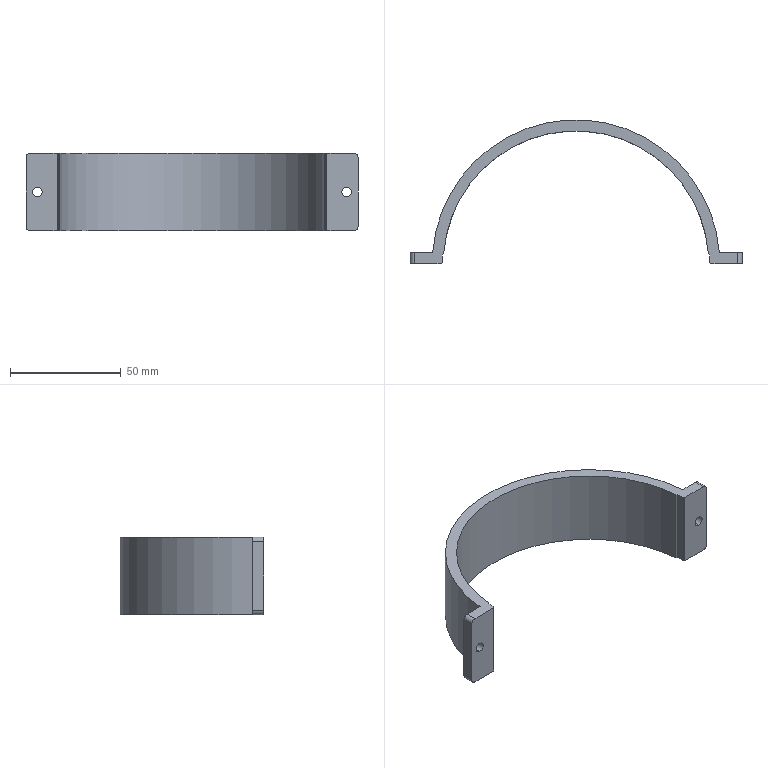Part | SolidWorks | features Chamfer 1, Extrusion 1, Fillet 1, HoleWzd 1, ICE 1 | 1 solid | 24 faces | box 150 x 64.95 x 35 mm | volume 37539 mm3 | cylinder 12 | plane 12 | commonest cylinder face diameters 4 x4 4.5 x4 120.9 x2 119.9 x1 129.9 x1
STEP:
#1=CARTESIAN_POINT('',(-69.879,0.,-2.25));
#2=VERTEX_POINT('',#1);
#3=CARTESIAN_POINT('',(-69.879,0.,2.25));
#4=VERTEX_POINT('',#3);
#5=CARTESIAN_POINT('',(-69.879,0.,0.));
#6=DIRECTION('',(0.,1.,0.));
#7=DIRECTION('',(0.,0.,1.));
#8=AXIS2_PLACEMENT_3D('',#5,#6,#7);
#9=CIRCLE('',#8,2.25);
#10=EDGE_CURVE('',#2,#4,#9,.T.);
#11=ORIENTED_EDGE('',*,*,#10,.F.);
#12=CARTESIAN_POINT('',(-69.879,5.,-2.25));
#13=VERTEX_POINT('',#12);
#14=CARTESIAN_POINT('',(-69.879,5.,-2.25));
#15=DIRECTION('',(0.,1.,0.));
#16=VECTOR('',#15,1000.);
#17=LINE('',#14,#16);
#18=EDGE_CURVE('',#2,#13,#17,.T.);
#19=ORIENTED_EDGE('',*,*,#18,.T.);
#20=CARTESIAN_POINT('',(-69.879,5.,2.25));
#21=VERTEX_POINT('',#20);
#22=CARTESIAN_POINT('',(-69.879,5.,0.));
#23=DIRECTION('',(0.,1.,0.));
#24=DIRECTION('',(0.,0.,1.));
#25=AXIS2_PLACEMENT_3D('',#22,#23,#24);
#26=CIRCLE('',#25,2.25);
#27=EDGE_CURVE('',#13,#21,#26,.T.);
#28=ORIENTED_EDGE('',*,*,#27,.T.);
#29=CARTESIAN_POINT('',(-69.879,5.,2.25));
#30=DIRECTION('',(0.,1.,0.));
#31=VECTOR('',#30,1000.);
#32=LINE('',#29,#31);
#33=EDGE_CURVE('',#4,#21,#32,.T.);
#34=ORIENTED_EDGE('',*,*,#33,.F.);
#35=EDGE_LOOP('',(#11,#19,#28,#34));
#36=FACE_OUTER_BOUND('',#35,.T.);
#37=CARTESIAN_POINT('',(-69.879,5.,0.));
#38=DIRECTION('',(0.,1.,0.));
#39=DIRECTION('',(0.,0.,1.));
#40=AXIS2_PLACEMENT_3D('',#37,#38,#39);
#41=CYLINDRICAL_SURFACE('',#40,2.25);
#42=ADVANCED_FACE('',(#36),#41,.F.);
#43=CARTESIAN_POINT('',(69.879,0.,-2.25));
#44=VERTEX_POINT('',#43);
#45=CARTESIAN_POINT('',(69.879,0.,2.25));
#46=VERTEX_POINT('',#45);
#47=CARTESIAN_POINT('',(69.879,0.,0.));
#48=DIRECTION('',(0.,1.,0.));
#49=DIRECTION('',(0.,0.,1.));
#50=AXIS2_PLACEMENT_3D('',#47,#48,#49);
#51=CIRCLE('',#50,2.25);
#52=EDGE_CURVE('',#44,#46,#51,.T.);
#53=ORIENTED_EDGE('',*,*,#52,.F.);
#54=CARTESIAN_POINT('',(69.879,5.,-2.25));
#55=VERTEX_POINT('',#54);
#56=CARTESIAN_POINT('',(69.879,5.,-2.25));
#57=DIRECTION('',(0.,1.,0.));
#58=VECTOR('',#57,1000.);
#59=LINE('',#56,#58);
#60=EDGE_CURVE('',#44,#55,#59,.T.);
#61=ORIENTED_EDGE('',*,*,#60,.T.);
#62=CARTESIAN_POINT('',(69.879,5.,2.25));
#63=VERTEX_POINT('',#62);
#64=CARTESIAN_POINT('',(69.879,5.,0.));
#65=DIRECTION('',(0.,1.,0.));
#66=DIRECTION('',(0.,0.,1.));
#67=AXIS2_PLACEMENT_3D('',#64,#65,#66);
#68=CIRCLE('',#67,2.25);
#69=EDGE_CURVE('',#55,#63,#68,.T.);
#70=ORIENTED_EDGE('',*,*,#69,.T.);
#71=CARTESIAN_POINT('',(69.879,5.,2.25));
#72=DIRECTION('',(0.,1.,0.));
#73=VECTOR('',#72,1000.);
#74=LINE('',#71,#73);
#75=EDGE_CURVE('',#46,#63,#74,.T.);
#76=ORIENTED_EDGE('',*,*,#75,.F.);
#77=EDGE_LOOP('',(#53,#61,#70,#76));
#78=FACE_OUTER_BOUND('',#77,.T.);
#79=CARTESIAN_POINT('',(69.879,5.,0.));
#80=DIRECTION('',(0.,1.,0.));
#81=DIRECTION('',(0.,0.,1.));
#82=AXIS2_PLACEMENT_3D('',#79,#80,#81);
#83=CYLINDRICAL_SURFACE('',#82,2.25);
#84=ADVANCED_FACE('',(#78),#83,.F.);
#85=CARTESIAN_POINT('',(64.757,5.,-17.5));
#86=VERTEX_POINT('',#85);
#87=CARTESIAN_POINT('',(-64.757,5.,-17.5));
#88=VERTEX_POINT('',#87);
#89=CARTESIAN_POINT('',(0.,0.,-17.5));
#90=DIRECTION('',(0.,0.,1.));
#91=DIRECTION('',(1.,0.,0.));
#92=AXIS2_PLACEMENT_3D('',#89,#90,#91);
#93=CIRCLE('',#92,64.95);
#94=EDGE_CURVE('',#86,#88,#93,.T.);
#95=ORIENTED_EDGE('',*,*,#94,.T.);
#96=CARTESIAN_POINT('',(-64.757,5.,17.5));
#97=VERTEX_POINT('',#96);
#98=CARTESIAN_POINT('',(-64.757,5.,17.5));
#99=DIRECTION('',(0.,0.,-1.));
#100=VECTOR('',#99,1000.);
#101=LINE('',#98,#100);
#102=EDGE_CURVE('',#97,#88,#101,.T.);
#103=ORIENTED_EDGE('',*,*,#102,.F.);
#104=CARTESIAN_POINT('',(64.757,5.,17.5));
#105=VERTEX_POINT('',#104);
#106=CARTESIAN_POINT('',(0.,0.,17.5));
#107=DIRECTION('',(0.,0.,1.));
#108=DIRECTION('',(1.,0.,0.));
#109=AXIS2_PLACEMENT_3D('',#106,#107,#108);
#110=CIRCLE('',#109,64.95);
#111=EDGE_CURVE('',#105,#97,#110,.T.);
#112=ORIENTED_EDGE('',*,*,#111,.F.);
#113=CARTESIAN_POINT('',(64.757,5.,17.5));
#114=DIRECTION('',(0.,0.,-1.));
#115=VECTOR('',#114,1000.);
#116=LINE('',#113,#115);
#117=EDGE_CURVE('',#105,#86,#116,.T.);
#118=ORIENTED_EDGE('',*,*,#117,.T.);
#119=EDGE_LOOP('',(#95,#103,#112,#118));
#120=FACE_OUTER_BOUND('',#119,.T.);
#121=CARTESIAN_POINT('',(0.,0.,17.5));
#122=DIRECTION('',(0.,0.,-1.));
#123=DIRECTION('',(-1.,0.,0.));
#124=AXIS2_PLACEMENT_3D('',#121,#122,#123);
#125=CYLINDRICAL_SURFACE('',#124,64.95);
#126=ADVANCED_FACE('',(#120),#125,.T.);
#127=CARTESIAN_POINT('',(-69.879,5.,0.));
#128=DIRECTION('',(0.,1.,0.));
#129=DIRECTION('',(0.,0.,1.));
#130=AXIS2_PLACEMENT_3D('',#127,#128,#129);
#131=CIRCLE('',#130,2.25);
#132=EDGE_CURVE('',#21,#13,#131,.T.);
#133=ORIENTED_EDGE('',*,*,#132,.F.);
#134=ORIENTED_EDGE('',*,*,#27,.F.);
#135=EDGE_LOOP('',(#133,#134));
#136=FACE_BOUND('',#135,.T.);
#137=CARTESIAN_POINT('',(-73.,5.,-17.5));
#138=VERTEX_POINT('',#137);
#139=CARTESIAN_POINT('',(-75.,5.,-17.5));
#140=DIRECTION('',(-1.,0.,0.));
#141=VECTOR('',#140,1000.);
#142=LINE('',#139,#141);
#143=EDGE_CURVE('',#88,#138,#142,.T.);
#144=ORIENTED_EDGE('',*,*,#143,.T.);
#145=CARTESIAN_POINT('',(-75.,5.,-15.5));
#146=VERTEX_POINT('',#145);
#147=CARTESIAN_POINT('',(-73.,5.,-15.5));
#148=DIRECTION('',(0.,1.,0.));
#149=DIRECTION('',(0.,0.,-1.));
#150=AXIS2_PLACEMENT_3D('',#147,#148,#149);
#151=CIRCLE('',#150,2.);
#152=EDGE_CURVE('',#138,#146,#151,.T.);
#153=ORIENTED_EDGE('',*,*,#152,.T.);
#154=CARTESIAN_POINT('',(-75.,5.,15.5));
#155=VERTEX_POINT('',#154);
#156=CARTESIAN_POINT('',(-75.,5.,17.5));
#157=DIRECTION('',(0.,0.,-1.));
#158=VECTOR('',#157,1000.);
#159=LINE('',#156,#158);
#160=EDGE_CURVE('',#155,#146,#159,.T.);
#161=ORIENTED_EDGE('',*,*,#160,.F.);
#162=CARTESIAN_POINT('',(-73.,5.,17.5));
#163=VERTEX_POINT('',#162);
#164=CARTESIAN_POINT('',(-73.,5.,15.5));
#165=DIRECTION('',(0.,1.,0.));
#166=DIRECTION('',(0.,0.,-1.));
#167=AXIS2_PLACEMENT_3D('',#164,#165,#166);
#168=CIRCLE('',#167,2.);
#169=EDGE_CURVE('',#155,#163,#168,.T.);
#170=ORIENTED_EDGE('',*,*,#169,.T.);
#171=CARTESIAN_POINT('',(-75.,5.,17.5));
#172=DIRECTION('',(-1.,0.,0.));
#173=VECTOR('',#172,1000.);
#174=LINE('',#171,#173);
#175=EDGE_CURVE('',#97,#163,#174,.T.);
#176=ORIENTED_EDGE('',*,*,#175,.F.);
#177=ORIENTED_EDGE('',*,*,#102,.T.);
#178=EDGE_LOOP('',(#144,#153,#161,#170,#176,#177));
#179=FACE_OUTER_BOUND('',#178,.T.);
#180=CARTESIAN_POINT('',(-75.,5.,17.5));
#181=DIRECTION('',(0.,-1.,0.));
#182=DIRECTION('',(0.,0.,-1.));
#183=AXIS2_PLACEMENT_3D('',#180,#181,#182);
#184=PLANE('',#183);
#185=ADVANCED_FACE('',(#136,#179),#184,.F.);
#186=ORIENTED_EDGE('',*,*,#160,.T.);
#187=CARTESIAN_POINT('',(-75.,0.,-15.5));
#188=VERTEX_POINT('',#187);
#189=CARTESIAN_POINT('',(-75.,0.,-15.5));
#190=DIRECTION('',(0.,-1.,0.));
#191=VECTOR('',#190,1000.);
#192=LINE('',#189,#191);
#193=EDGE_CURVE('',#146,#188,#192,.T.);
#194=ORIENTED_EDGE('',*,*,#193,.T.);
#195=CARTESIAN_POINT('',(-75.,0.,15.5));
#196=VERTEX_POINT('',#195);
#197=CARTESIAN_POINT('',(-75.,0.,17.5));
#198=DIRECTION('',(0.,0.,-1.));
#199=VECTOR('',#198,1000.);
#200=LINE('',#197,#199);
#201=EDGE_CURVE('',#196,#188,#200,.T.);
#202=ORIENTED_EDGE('',*,*,#201,.F.);
#203=CARTESIAN_POINT('',(-75.,5.,15.5));
#204=DIRECTION('',(0.,1.,0.));
#205=VECTOR('',#204,1000.);
#206=LINE('',#203,#205);
#207=EDGE_CURVE('',#196,#155,#206,.T.);
#208=ORIENTED_EDGE('',*,*,#207,.T.);
#209=EDGE_LOOP('',(#186,#194,#202,#208));
#210=FACE_OUTER_BOUND('',#209,.T.);
#211=CARTESIAN_POINT('',(-75.,0.,17.5));
#212=DIRECTION('',(1.,0.,0.));
#213=DIRECTION('',(0.,0.,-1.));
#214=AXIS2_PLACEMENT_3D('',#211,#212,#213);
#215=PLANE('',#214);
#216=ADVANCED_FACE('',(#210),#215,.F.);
#217=CARTESIAN_POINT('',(-69.879,0.,0.));
#218=DIRECTION('',(0.,1.,0.));
#219=DIRECTION('',(0.,0.,1.));
#220=AXIS2_PLACEMENT_3D('',#217,#218,#219);
#221=CIRCLE('',#220,2.25);
#222=EDGE_CURVE('',#4,#2,#221,.T.);
#223=ORIENTED_EDGE('',*,*,#222,.T.);
#224=ORIENTED_EDGE('',*,*,#10,.T.);
#225=EDGE_LOOP('',(#223,#224));
#226=FACE_BOUND('',#225,.T.);
#227=CARTESIAN_POINT('',(-73.,0.,-17.5));
#228=VERTEX_POINT('',#227);
#229=CARTESIAN_POINT('',(-60.95,0.,-17.5));
#230=VERTEX_POINT('',#229);
#231=CARTESIAN_POINT('',(-59.95,0.,-17.5));
#232=DIRECTION('',(1.,0.,0.));
#233=VECTOR('',#232,1000.);
#234=LINE('',#231,#233);
#235=EDGE_CURVE('',#228,#230,#234,.T.);
#236=ORIENTED_EDGE('',*,*,#235,.T.);
#237=CARTESIAN_POINT('',(-60.95,0.,17.5));
#238=VERTEX_POINT('',#237);
#239=CARTESIAN_POINT('',(-60.95,0.,17.5));
#240=DIRECTION('',(0.,0.,1.));
#241=VECTOR('',#240,1000.);
#242=LINE('',#239,#241);
#243=EDGE_CURVE('',#230,#238,#242,.T.);
#244=ORIENTED_EDGE('',*,*,#243,.T.);
#245=CARTESIAN_POINT('',(-73.,0.,17.5));
#246=VERTEX_POINT('',#245);
#247=CARTESIAN_POINT('',(-59.95,0.,17.5));
#248=DIRECTION('',(1.,0.,0.));
#249=VECTOR('',#248,1000.);
#250=LINE('',#247,#249);
#251=EDGE_CURVE('',#246,#238,#250,.T.);
#252=ORIENTED_EDGE('',*,*,#251,.F.);
#253=CARTESIAN_POINT('',(-73.,0.,15.5));
#254=DIRECTION('',(0.,-1.,0.));
#255=DIRECTION('',(0.,0.,1.));
#256=AXIS2_PLACEMENT_3D('',#253,#254,#255);
#257=CIRCLE('',#256,2.);
#258=EDGE_CURVE('',#246,#196,#257,.T.);
#259=ORIENTED_EDGE('',*,*,#258,.T.);
#260=ORIENTED_EDGE('',*,*,#201,.T.);
#261=CARTESIAN_POINT('',(-73.,0.,-15.5));
#262=DIRECTION('',(0.,-1.,0.));
#263=DIRECTION('',(0.,0.,1.));
#264=AXIS2_PLACEMENT_3D('',#261,#262,#263);
#265=CIRCLE('',#264,2.);
#266=EDGE_CURVE('',#188,#228,#265,.T.);
#267=ORIENTED_EDGE('',*,*,#266,.T.);
#268=EDGE_LOOP('',(#236,#244,#252,#259,#260,#267));
#269=FACE_OUTER_BOUND('',#268,.T.);
#270=CARTESIAN_POINT('',(-59.95,0.,17.5));
#271=DIRECTION('',(0.,1.,0.));
#272=DIRECTION('',(0.,0.,1.));
#273=AXIS2_PLACEMENT_3D('',#270,#271,#272);
#274=PLANE('',#273);
#275=ADVANCED_FACE('',(#226,#269),#274,.F.);
#276=CARTESIAN_POINT('',(-59.781,4.494,17.5));
#277=VERTEX_POINT('',#276);
#278=CARTESIAN_POINT('',(59.781,4.494,17.5));
#279=VERTEX_POINT('',#278);
#280=CARTESIAN_POINT('',(0.,0.,17.5));
#281=DIRECTION('',(0.,0.,-1.));
#282=DIRECTION('',(1.,0.,0.));
#283=AXIS2_PLACEMENT_3D('',#280,#281,#282);
#284=CIRCLE('',#283,59.95);
#285=EDGE_CURVE('',#277,#279,#284,.T.);
#286=ORIENTED_EDGE('',*,*,#285,.F.);
#287=CARTESIAN_POINT('',(-59.781,4.494,-17.5));
#288=VERTEX_POINT('',#287);
#289=CARTESIAN_POINT('',(-59.781,4.494,17.5));
#290=DIRECTION('',(0.,0.,-1.));
#291=VECTOR('',#290,1000.);
#292=LINE('',#289,#291);
#293=EDGE_CURVE('',#277,#288,#292,.T.);
#294=ORIENTED_EDGE('',*,*,#293,.T.);
#295=CARTESIAN_POINT('',(59.781,4.494,-17.5));
#296=VERTEX_POINT('',#295);
#297=CARTESIAN_POINT('',(0.,0.,-17.5));
#298=DIRECTION('',(0.,0.,-1.));
#299=DIRECTION('',(1.,0.,0.));
#300=AXIS2_PLACEMENT_3D('',#297,#298,#299);
#301=CIRCLE('',#300,59.95);
#302=EDGE_CURVE('',#288,#296,#301,.T.);
#303=ORIENTED_EDGE('',*,*,#302,.T.);
#304=CARTESIAN_POINT('',(59.781,4.494,17.5));
#305=DIRECTION('',(0.,0.,1.));
#306=VECTOR('',#305,1000.);
#307=LINE('',#304,#306);
#308=EDGE_CURVE('',#296,#279,#307,.T.);
#309=ORIENTED_EDGE('',*,*,#308,.T.);
#310=EDGE_LOOP('',(#286,#294,#303,#309));
#311=FACE_OUTER_BOUND('',#310,.T.);
#312=CARTESIAN_POINT('',(0.,0.,17.5));
#313=DIRECTION('',(0.,0.,-1.));
#314=DIRECTION('',(-1.,0.,0.));
#315=AXIS2_PLACEMENT_3D('',#312,#313,#314);
#316=CYLINDRICAL_SURFACE('',#315,59.95);
#317=ADVANCED_FACE('',(#311),#316,.F.);
#318=CARTESIAN_POINT('',(69.879,0.,0.));
#319=DIRECTION('',(0.,1.,0.));
#320=DIRECTION('',(0.,0.,1.));
#321=AXIS2_PLACEMENT_3D('',#318,#319,#320);
#322=CIRCLE('',#321,2.25);
#323=EDGE_CURVE('',#46,#44,#322,.T.);
#324=ORIENTED_EDGE('',*,*,#323,.T.);
#325=ORIENTED_EDGE('',*,*,#52,.T.);
#326=EDGE_LOOP('',(#324,#325));
#327=FACE_BOUND('',#326,.T.);
#328=CARTESIAN_POINT('',(60.95,0.,17.5));
#329=VERTEX_POINT('',#328);
#330=CARTESIAN_POINT('',(73.,0.,17.5));
#331=VERTEX_POINT('',#330);
#332=CARTESIAN_POINT('',(75.,0.,17.5));
#333=DIRECTION('',(1.,0.,0.));
#334=VECTOR('',#333,1000.);
#335=LINE('',#332,#334);
#336=EDGE_CURVE('',#329,#331,#335,.T.);
#337=ORIENTED_EDGE('',*,*,#336,.F.);
#338=CARTESIAN_POINT('',(60.95,0.,-17.5));
#339=VERTEX_POINT('',#338);
#340=CARTESIAN_POINT('',(60.95,0.,17.5));
#341=DIRECTION('',(0.,0.,-1.));
#342=VECTOR('',#341,1000.);
#343=LINE('',#340,#342);
#344=EDGE_CURVE('',#329,#339,#343,.T.);
#345=ORIENTED_EDGE('',*,*,#344,.T.);
#346=CARTESIAN_POINT('',(73.,0.,-17.5));
#347=VERTEX_POINT('',#346);
#348=CARTESIAN_POINT('',(75.,0.,-17.5));
#349=DIRECTION('',(1.,0.,0.));
#350=VECTOR('',#349,1000.);
#351=LINE('',#348,#350);
#352=EDGE_CURVE('',#339,#347,#351,.T.);
#353=ORIENTED_EDGE('',*,*,#352,.T.);
#354=CARTESIAN_POINT('',(75.,0.,-15.5));
#355=VERTEX_POINT('',#354);
#356=CARTESIAN_POINT('',(73.,0.,-15.5));
#357=DIRECTION('',(0.,-1.,0.));
#358=DIRECTION('',(0.,0.,1.));
#359=AXIS2_PLACEMENT_3D('',#356,#357,#358);
#360=CIRCLE('',#359,2.);
#361=EDGE_CURVE('',#347,#355,#360,.T.);
#362=ORIENTED_EDGE('',*,*,#361,.T.);
#363=CARTESIAN_POINT('',(75.,0.,15.5));
#364=VERTEX_POINT('',#363);
#365=CARTESIAN_POINT('',(75.,0.,17.5));
#366=DIRECTION('',(0.,0.,-1.));
#367=VECTOR('',#366,1000.);
#368=LINE('',#365,#367);
#369=EDGE_CURVE('',#364,#355,#368,.T.);
#370=ORIENTED_EDGE('',*,*,#369,.F.);
#371=CARTESIAN_POINT('',(73.,0.,15.5));
#372=DIRECTION('',(0.,-1.,0.));
#373=DIRECTION('',(0.,0.,1.));
#374=AXIS2_PLACEMENT_3D('',#371,#372,#373);
#375=CIRCLE('',#374,2.);
#376=EDGE_CURVE('',#364,#331,#375,.T.);
#377=ORIENTED_EDGE('',*,*,#376,.T.);
#378=EDGE_LOOP('',(#337,#345,#353,#362,#370,#377));
#379=FACE_OUTER_BOUND('',#378,.T.);
#380=CARTESIAN_POINT('',(75.,0.,17.5));
#381=DIRECTION('',(0.,1.,0.));
#382=DIRECTION('',(0.,0.,1.));
#383=AXIS2_PLACEMENT_3D('',#380,#381,#382);
#384=PLANE('',#383);
#385=ADVANCED_FACE('',(#327,#379),#384,.F.);
#386=ORIENTED_EDGE('',*,*,#369,.T.);
#387=CARTESIAN_POINT('',(75.,5.,-15.5));
#388=VERTEX_POINT('',#387);
#389=CARTESIAN_POINT('',(75.,5.,-15.5));
#390=DIRECTION('',(0.,1.,0.));
#391=VECTOR('',#390,1000.);
#392=LINE('',#389,#391);
#393=EDGE_CURVE('',#355,#388,#392,.T.);
#394=ORIENTED_EDGE('',*,*,#393,.T.);
#395=CARTESIAN_POINT('',(75.,5.,15.5));
#396=VERTEX_POINT('',#395);
#397=CARTESIAN_POINT('',(75.,5.,17.5));
#398=DIRECTION('',(0.,0.,-1.));
#399=VECTOR('',#398,1000.);
#400=LINE('',#397,#399);
#401=EDGE_CURVE('',#396,#388,#400,.T.);
#402=ORIENTED_EDGE('',*,*,#401,.F.);
#403=CARTESIAN_POINT('',(75.,0.,15.5));
#404=DIRECTION('',(0.,-1.,0.));
#405=VECTOR('',#404,1000.);
#406=LINE('',#403,#405);
#407=EDGE_CURVE('',#396,#364,#406,.T.);
#408=ORIENTED_EDGE('',*,*,#407,.T.);
#409=EDGE_LOOP('',(#386,#394,#402,#408));
#410=FACE_OUTER_BOUND('',#409,.T.);
#411=CARTESIAN_POINT('',(75.,5.,17.5));
#412=DIRECTION('',(-1.,0.,0.));
#413=DIRECTION('',(0.,0.,1.));
#414=AXIS2_PLACEMENT_3D('',#411,#412,#413);
#415=PLANE('',#414);
#416=ADVANCED_FACE('',(#410),#415,.F.);
#417=CARTESIAN_POINT('',(69.879,5.,0.));
#418=DIRECTION('',(0.,1.,0.));
#419=DIRECTION('',(0.,0.,1.));
#420=AXIS2_PLACEMENT_3D('',#417,#418,#419);
#421=CIRCLE('',#420,2.25);
#422=EDGE_CURVE('',#63,#55,#421,.T.);
#423=ORIENTED_EDGE('',*,*,#422,.F.);
#424=ORIENTED_EDGE('',*,*,#69,.F.);
#425=EDGE_LOOP('',(#423,#424));
#426=FACE_BOUND('',#425,.T.);
#427=ORIENTED_EDGE('',*,*,#401,.T.);
#428=CARTESIAN_POINT('',(73.,5.,-17.5));
#429=VERTEX_POINT('',#428);
#430=CARTESIAN_POINT('',(73.,5.,-15.5));
#431=DIRECTION('',(0.,1.,0.));
#432=DIRECTION('',(1.,0.,0.));
#433=AXIS2_PLACEMENT_3D('',#430,#431,#432);
#434=CIRCLE('',#433,2.);
#435=EDGE_CURVE('',#388,#429,#434,.T.);
#436=ORIENTED_EDGE('',*,*,#435,.T.);
#437=CARTESIAN_POINT('',(64.757,5.,-17.5));
#438=DIRECTION('',(-1.,0.,0.));
#439=VECTOR('',#438,1000.);
#440=LINE('',#437,#439);
#441=EDGE_CURVE('',#429,#86,#440,.T.);
#442=ORIENTED_EDGE('',*,*,#441,.T.);
#443=ORIENTED_EDGE('',*,*,#117,.F.);
#444=CARTESIAN_POINT('',(73.,5.,17.5));
#445=VERTEX_POINT('',#444);
#446=CARTESIAN_POINT('',(64.757,5.,17.5));
#447=DIRECTION('',(-1.,0.,0.));
#448=VECTOR('',#447,1000.);
#449=LINE('',#446,#448);
#450=EDGE_CURVE('',#445,#105,#449,.T.);
#451=ORIENTED_EDGE('',*,*,#450,.F.);
#452=CARTESIAN_POINT('',(73.,5.,15.5));
#453=DIRECTION('',(0.,1.,0.));
#454=DIRECTION('',(1.,0.,0.));
#455=AXIS2_PLACEMENT_3D('',#452,#453,#454);
#456=CIRCLE('',#455,2.);
#457=EDGE_CURVE('',#445,#396,#456,.T.);
#458=ORIENTED_EDGE('',*,*,#457,.T.);
#459=EDGE_LOOP('',(#427,#436,#442,#443,#451,#458));
#460=FACE_OUTER_BOUND('',#459,.T.);
#461=CARTESIAN_POINT('',(64.757,5.,17.5));
#462=DIRECTION('',(0.,-1.,0.));
#463=DIRECTION('',(1.,0.,0.));
#464=AXIS2_PLACEMENT_3D('',#461,#462,#463);
#465=PLANE('',#464);
#466=ADVANCED_FACE('',(#426,#460),#465,.F.);
#467=CARTESIAN_POINT('',(-60.315,4.031,17.5));
#468=VERTEX_POINT('',#467);
#469=CARTESIAN_POINT('',(-60.448,0.5021,17.5));
#470=VERTEX_POINT('',#469);
#471=CARTESIAN_POINT('',(0.,0.,17.5));
#472=DIRECTION('',(0.,0.,1.));
#473=DIRECTION('',(1.,0.,0.));
#474=AXIS2_PLACEMENT_3D('',#471,#472,#473);
#475=CIRCLE('',#474,60.45);
#476=EDGE_CURVE('',#468,#470,#475,.T.);
#477=ORIENTED_EDGE('',*,*,#476,.F.);
#478=CARTESIAN_POINT('',(-27.874,32.154,17.5));
#479=DIRECTION('',(0.7556,0.655,0.));
#480=VECTOR('',#479,1000.);
#481=LINE('',#478,#480);
#482=EDGE_CURVE('',#468,#277,#481,.T.);
#483=ORIENTED_EDGE('',*,*,#482,.T.);
#484=ORIENTED_EDGE('',*,*,#285,.T.);
#485=CARTESIAN_POINT('',(60.315,4.031,17.5));
#486=VERTEX_POINT('',#485);
#487=CARTESIAN_POINT('',(27.874,32.154,17.5));
#488=DIRECTION('',(0.7556,-0.655,0.));
#489=VECTOR('',#488,1000.);
#490=LINE('',#487,#489);
#491=EDGE_CURVE('',#279,#486,#490,.T.);
#492=ORIENTED_EDGE('',*,*,#491,.T.);
#493=CARTESIAN_POINT('',(60.448,0.5021,17.5));
#494=VERTEX_POINT('',#493);
#495=CARTESIAN_POINT('',(0.,0.,17.5));
#496=DIRECTION('',(0.,0.,1.));
#497=DIRECTION('',(1.,0.,0.));
#498=AXIS2_PLACEMENT_3D('',#495,#496,#497);
#499=CIRCLE('',#498,60.45);
#500=EDGE_CURVE('',#494,#486,#499,.T.);
#501=ORIENTED_EDGE('',*,*,#500,.F.);
#502=CARTESIAN_POINT('',(30.475,30.475,17.5));
#503=DIRECTION('',(0.7071,-0.7071,0.));
#504=VECTOR('',#503,1000.);
#505=LINE('',#502,#504);
#506=EDGE_CURVE('',#494,#329,#505,.T.);
#507=ORIENTED_EDGE('',*,*,#506,.T.);
#508=ORIENTED_EDGE('',*,*,#336,.T.);
#509=CARTESIAN_POINT('',(73.,5.,17.5));
#510=DIRECTION('',(0.,1.,0.));
#511=VECTOR('',#510,1000.);
#512=LINE('',#509,#511);
#513=EDGE_CURVE('',#331,#445,#512,.T.);
#514=ORIENTED_EDGE('',*,*,#513,.T.);
#515=ORIENTED_EDGE('',*,*,#450,.T.);
#516=ORIENTED_EDGE('',*,*,#111,.T.);
#517=ORIENTED_EDGE('',*,*,#175,.T.);
#518=CARTESIAN_POINT('',(-73.,0.,17.5));
#519=DIRECTION('',(0.,-1.,0.));
#520=VECTOR('',#519,1000.);
#521=LINE('',#518,#520);
#522=EDGE_CURVE('',#163,#246,#521,.T.);
#523=ORIENTED_EDGE('',*,*,#522,.T.);
#524=ORIENTED_EDGE('',*,*,#251,.T.);
#525=CARTESIAN_POINT('',(-30.475,30.475,17.5));
#526=DIRECTION('',(0.7071,0.7071,0.));
#527=VECTOR('',#526,1000.);
#528=LINE('',#525,#527);
#529=EDGE_CURVE('',#238,#470,#528,.T.);
#530=ORIENTED_EDGE('',*,*,#529,.T.);
#531=EDGE_LOOP('',(#477,#483,#484,#492,#501,#507,#508,#514,#515,#516,#517,#523,#524,#530));
#532=FACE_OUTER_BOUND('',#531,.T.);
#533=CARTESIAN_POINT('',(0.,0.,17.5));
#534=DIRECTION('',(0.,0.,1.));
#535=DIRECTION('',(1.,0.,0.));
#536=AXIS2_PLACEMENT_3D('',#533,#534,#535);
#537=PLANE('',#536);
#538=ADVANCED_FACE('',(#532),#537,.T.);
#539=CARTESIAN_POINT('',(-60.315,4.031,-17.5));
#540=VERTEX_POINT('',#539);
#541=CARTESIAN_POINT('',(-60.351,4.,-17.5));
#542=DIRECTION('',(-0.7556,-0.655,0.));
#543=VECTOR('',#542,1000.);
#544=LINE('',#541,#543);
#545=EDGE_CURVE('',#288,#540,#544,.T.);
#546=ORIENTED_EDGE('',*,*,#545,.T.);
#547=CARTESIAN_POINT('',(-60.448,0.5021,-17.5));
#548=VERTEX_POINT('',#547);
#549=CARTESIAN_POINT('',(0.,0.,-17.5));
#550=DIRECTION('',(0.,0.,1.));
#551=DIRECTION('',(1.,0.,0.));
#552=AXIS2_PLACEMENT_3D('',#549,#550,#551);
#553=CIRCLE('',#552,60.45);
#554=EDGE_CURVE('',#540,#548,#553,.T.);
#555=ORIENTED_EDGE('',*,*,#554,.T.);
#556=CARTESIAN_POINT('',(-60.95,0.,-17.5));
#557=DIRECTION('',(-0.7071,-0.7071,0.));
#558=VECTOR('',#557,1000.);
#559=LINE('',#556,#558);
#560=EDGE_CURVE('',#548,#230,#559,.T.);
#561=ORIENTED_EDGE('',*,*,#560,.T.);
#562=ORIENTED_EDGE('',*,*,#235,.F.);
#563=CARTESIAN_POINT('',(-73.,0.,-17.5));
#564=DIRECTION('',(0.,1.,0.));
#565=VECTOR('',#564,1000.);
#566=LINE('',#563,#565);
#567=EDGE_CURVE('',#228,#138,#566,.T.);
#568=ORIENTED_EDGE('',*,*,#567,.T.);
#569=ORIENTED_EDGE('',*,*,#143,.F.);
#570=ORIENTED_EDGE('',*,*,#94,.F.);
#571=ORIENTED_EDGE('',*,*,#441,.F.);
#572=CARTESIAN_POINT('',(73.,0.,-17.5));
#573=DIRECTION('',(0.,-1.,0.));
#574=VECTOR('',#573,1000.);
#575=LINE('',#572,#574);
#576=EDGE_CURVE('',#429,#347,#575,.T.);
#577=ORIENTED_EDGE('',*,*,#576,.T.);
#578=ORIENTED_EDGE('',*,*,#352,.F.);
#579=CARTESIAN_POINT('',(60.448,0.5021,-17.5));
#580=VERTEX_POINT('',#579);
#581=CARTESIAN_POINT('',(60.448,0.5021,-17.5));
#582=DIRECTION('',(-0.7071,0.7071,0.));
#583=VECTOR('',#582,1000.);
#584=LINE('',#581,#583);
#585=EDGE_CURVE('',#339,#580,#584,.T.);
#586=ORIENTED_EDGE('',*,*,#585,.T.);
#587=CARTESIAN_POINT('',(60.315,4.031,-17.5));
#588=VERTEX_POINT('',#587);
#589=CARTESIAN_POINT('',(0.,0.,-17.5));
#590=DIRECTION('',(0.,0.,1.));
#591=DIRECTION('',(1.,0.,0.));
#592=AXIS2_PLACEMENT_3D('',#589,#590,#591);
#593=CIRCLE('',#592,60.45);
#594=EDGE_CURVE('',#580,#588,#593,.T.);
#595=ORIENTED_EDGE('',*,*,#594,.T.);
#596=CARTESIAN_POINT('',(59.781,4.494,-17.5));
#597=DIRECTION('',(-0.7556,0.655,0.));
#598=VECTOR('',#597,1000.);
#599=LINE('',#596,#598);
#600=EDGE_CURVE('',#588,#296,#599,.T.);
#601=ORIENTED_EDGE('',*,*,#600,.T.);
#602=ORIENTED_EDGE('',*,*,#302,.F.);
#603=EDGE_LOOP('',(#546,#555,#561,#562,#568,#569,#570,#571,#577,#578,#586,#595,#601,#602));
#604=FACE_OUTER_BOUND('',#603,.T.);
#605=CARTESIAN_POINT('',(0.,0.,-17.5));
#606=DIRECTION('',(0.,0.,1.));
#607=DIRECTION('',(1.,0.,0.));
#608=AXIS2_PLACEMENT_3D('',#605,#606,#607);
#609=PLANE('',#608);
#610=ADVANCED_FACE('',(#604),#609,.F.);
#611=ORIENTED_EDGE('',*,*,#60,.F.);
#612=ORIENTED_EDGE('',*,*,#323,.F.);
#613=ORIENTED_EDGE('',*,*,#75,.T.);
#614=ORIENTED_EDGE('',*,*,#422,.T.);
#615=EDGE_LOOP('',(#611,#612,#613,#614));
#616=FACE_OUTER_BOUND('',#615,.T.);
#617=CARTESIAN_POINT('',(69.879,5.,0.));
#618=DIRECTION('',(0.,1.,0.));
#619=DIRECTION('',(0.,0.,1.));
#620=AXIS2_PLACEMENT_3D('',#617,#618,#619);
#621=CYLINDRICAL_SURFACE('',#620,2.25);
#622=ADVANCED_FACE('',(#616),#621,.F.);
#623=ORIENTED_EDGE('',*,*,#18,.F.);
#624=ORIENTED_EDGE('',*,*,#222,.F.);
#625=ORIENTED_EDGE('',*,*,#33,.T.);
#626=ORIENTED_EDGE('',*,*,#132,.T.);
#627=EDGE_LOOP('',(#623,#624,#625,#626));
#628=FACE_OUTER_BOUND('',#627,.T.);
#629=CARTESIAN_POINT('',(-69.879,5.,0.));
#630=DIRECTION('',(0.,1.,0.));
#631=DIRECTION('',(0.,0.,1.));
#632=AXIS2_PLACEMENT_3D('',#629,#630,#631);
#633=CYLINDRICAL_SURFACE('',#632,2.25);
#634=ADVANCED_FACE('',(#628),#633,.F.);
#635=ORIENTED_EDGE('',*,*,#361,.F.);
#636=ORIENTED_EDGE('',*,*,#576,.F.);
#637=ORIENTED_EDGE('',*,*,#435,.F.);
#638=ORIENTED_EDGE('',*,*,#393,.F.);
#639=EDGE_LOOP('',(#635,#636,#637,#638));
#640=FACE_OUTER_BOUND('',#639,.T.);
#641=CARTESIAN_POINT('',(73.,5.,-15.5));
#642=DIRECTION('',(0.,1.,0.));
#643=DIRECTION('',(0.,0.,1.));
#644=AXIS2_PLACEMENT_3D('',#641,#642,#643);
#645=CYLINDRICAL_SURFACE('',#644,2.);
#646=ADVANCED_FACE('',(#640),#645,.T.);
#647=ORIENTED_EDGE('',*,*,#376,.F.);
#648=ORIENTED_EDGE('',*,*,#407,.F.);
#649=ORIENTED_EDGE('',*,*,#457,.F.);
#650=ORIENTED_EDGE('',*,*,#513,.F.);
#651=EDGE_LOOP('',(#647,#648,#649,#650));
#652=FACE_OUTER_BOUND('',#651,.T.);
#653=CARTESIAN_POINT('',(73.,0.,15.5));
#654=DIRECTION('',(0.,-1.,0.));
#655=DIRECTION('',(0.,0.,-1.));
#656=AXIS2_PLACEMENT_3D('',#653,#654,#655);
#657=CYLINDRICAL_SURFACE('',#656,2.);
#658=ADVANCED_FACE('',(#652),#657,.T.);
#659=ORIENTED_EDGE('',*,*,#152,.F.);
#660=ORIENTED_EDGE('',*,*,#567,.F.);
#661=ORIENTED_EDGE('',*,*,#266,.F.);
#662=ORIENTED_EDGE('',*,*,#193,.F.);
#663=EDGE_LOOP('',(#659,#660,#661,#662));
#664=FACE_OUTER_BOUND('',#663,.T.);
#665=CARTESIAN_POINT('',(-73.,0.,-15.5));
#666=DIRECTION('',(0.,-1.,0.));
#667=DIRECTION('',(0.,0.,-1.));
#668=AXIS2_PLACEMENT_3D('',#665,#666,#667);
#669=CYLINDRICAL_SURFACE('',#668,2.);
#670=ADVANCED_FACE('',(#664),#669,.T.);
#671=ORIENTED_EDGE('',*,*,#169,.F.);
#672=ORIENTED_EDGE('',*,*,#207,.F.);
#673=ORIENTED_EDGE('',*,*,#258,.F.);
#674=ORIENTED_EDGE('',*,*,#522,.F.);
#675=EDGE_LOOP('',(#671,#672,#673,#674));
#676=FACE_OUTER_BOUND('',#675,.T.);
#677=CARTESIAN_POINT('',(-73.,0.,15.5));
#678=DIRECTION('',(0.,1.,0.));
#679=DIRECTION('',(0.,0.,1.));
#680=AXIS2_PLACEMENT_3D('',#677,#678,#679);
#681=CYLINDRICAL_SURFACE('',#680,2.);
#682=ADVANCED_FACE('',(#676),#681,.T.);
#683=ORIENTED_EDGE('',*,*,#594,.F.);
#684=CARTESIAN_POINT('',(60.448,0.5021,-17.5));
#685=DIRECTION('',(0.,0.,1.));
#686=VECTOR('',#685,1000.);
#687=LINE('',#684,#686);
#688=EDGE_CURVE('',#580,#494,#687,.T.);
#689=ORIENTED_EDGE('',*,*,#688,.T.);
#690=ORIENTED_EDGE('',*,*,#500,.T.);
#691=CARTESIAN_POINT('',(60.315,4.031,0.));
#692=DIRECTION('',(0.,0.,-1.));
#693=VECTOR('',#692,1000.);
#694=LINE('',#691,#693);
#695=EDGE_CURVE('',#486,#588,#694,.T.);
#696=ORIENTED_EDGE('',*,*,#695,.T.);
#697=EDGE_LOOP('',(#683,#689,#690,#696));
#698=FACE_OUTER_BOUND('',#697,.T.);
#699=CARTESIAN_POINT('',(0.,0.,-17.5));
#700=DIRECTION('',(0.,0.,1.));
#701=DIRECTION('',(1.,0.,0.));
#702=AXIS2_PLACEMENT_3D('',#699,#700,#701);
#703=CYLINDRICAL_SURFACE('',#702,60.45);
#704=ADVANCED_FACE('',(#698),#703,.F.);
#705=ORIENTED_EDGE('',*,*,#476,.T.);
#706=CARTESIAN_POINT('',(-60.448,0.5021,-17.5));
#707=DIRECTION('',(0.,0.,-1.));
#708=VECTOR('',#707,1000.);
#709=LINE('',#706,#708);
#710=EDGE_CURVE('',#470,#548,#709,.T.);
#711=ORIENTED_EDGE('',*,*,#710,.T.);
#712=ORIENTED_EDGE('',*,*,#554,.F.);
#713=CARTESIAN_POINT('',(-60.315,4.031,0.));
#714=DIRECTION('',(0.,0.,1.));
#715=VECTOR('',#714,1000.);
#716=LINE('',#713,#715);
#717=EDGE_CURVE('',#540,#468,#716,.T.);
#718=ORIENTED_EDGE('',*,*,#717,.T.);
#719=EDGE_LOOP('',(#705,#711,#712,#718));
#720=FACE_OUTER_BOUND('',#719,.T.);
#721=CARTESIAN_POINT('',(0.,0.,-17.5));
#722=DIRECTION('',(0.,0.,1.));
#723=DIRECTION('',(1.,0.,0.));
#724=AXIS2_PLACEMENT_3D('',#721,#722,#723);
#725=CYLINDRICAL_SURFACE('',#724,60.45);
#726=ADVANCED_FACE('',(#720),#725,.F.);
#727=ORIENTED_EDGE('',*,*,#545,.F.);
#728=ORIENTED_EDGE('',*,*,#293,.F.);
#729=ORIENTED_EDGE('',*,*,#482,.F.);
#730=ORIENTED_EDGE('',*,*,#717,.F.);
#731=EDGE_LOOP('',(#727,#728,#729,#730));
#732=FACE_OUTER_BOUND('',#731,.T.);
#733=CARTESIAN_POINT('',(-60.351,4.,17.5));
#734=DIRECTION('',(0.655,-0.7556,0.));
#735=DIRECTION('',(0.,0.,-1.));
#736=AXIS2_PLACEMENT_3D('',#733,#734,#735);
#737=PLANE('',#736);
#738=ADVANCED_FACE('',(#732),#737,.T.);
#739=ORIENTED_EDGE('',*,*,#585,.F.);
#740=ORIENTED_EDGE('',*,*,#344,.F.);
#741=ORIENTED_EDGE('',*,*,#506,.F.);
#742=ORIENTED_EDGE('',*,*,#688,.F.);
#743=EDGE_LOOP('',(#739,#740,#741,#742));
#744=FACE_OUTER_BOUND('',#743,.T.);
#745=CARTESIAN_POINT('',(60.448,0.5021,-17.5));
#746=DIRECTION('',(0.7071,0.7071,0.));
#747=DIRECTION('',(0.,0.,1.));
#748=AXIS2_PLACEMENT_3D('',#745,#746,#747);
#749=PLANE('',#748);
#750=ADVANCED_FACE('',(#744),#749,.F.);
#751=ORIENTED_EDGE('',*,*,#600,.F.);
#752=ORIENTED_EDGE('',*,*,#695,.F.);
#753=ORIENTED_EDGE('',*,*,#491,.F.);
#754=ORIENTED_EDGE('',*,*,#308,.F.);
#755=EDGE_LOOP('',(#751,#752,#753,#754));
#756=FACE_OUTER_BOUND('',#755,.T.);
#757=CARTESIAN_POINT('',(59.781,4.494,17.5));
#758=DIRECTION('',(-0.655,-0.7556,0.));
#759=DIRECTION('',(0.,0.,-1.));
#760=AXIS2_PLACEMENT_3D('',#757,#758,#759);
#761=PLANE('',#760);
#762=ADVANCED_FACE('',(#756),#761,.T.);
#763=ORIENTED_EDGE('',*,*,#560,.F.);
#764=ORIENTED_EDGE('',*,*,#710,.F.);
#765=ORIENTED_EDGE('',*,*,#529,.F.);
#766=ORIENTED_EDGE('',*,*,#243,.F.);
#767=EDGE_LOOP('',(#763,#764,#765,#766));
#768=FACE_OUTER_BOUND('',#767,.T.);
#769=CARTESIAN_POINT('',(-60.95,0.,-17.5));
#770=DIRECTION('',(-0.7071,0.7071,0.));
#771=DIRECTION('',(0.,0.,1.));
#772=AXIS2_PLACEMENT_3D('',#769,#770,#771);
#773=PLANE('',#772);
#774=ADVANCED_FACE('',(#768),#773,.F.);
#775=CLOSED_SHELL('',(#42,#84,#126,#185,#216,#275,#317,#385,#416,#466,#538,#610,#622,#634,#646,#658,#670,#682,#704,#726,#738,#750,#762,#774));
#776=MANIFOLD_SOLID_BREP('',#775);
#777=CARTESIAN_POINT('',(0.,0.,0.));
#778=DIRECTION('',(0.,0.,1.));
#779=DIRECTION('',(1.,0.,0.));
#780=AXIS2_PLACEMENT_3D('',#777,#778,#779);
#781=(LENGTH_UNIT()NAMED_UNIT(*)SI_UNIT(.MILLI.,.METRE.));
#782=UNCERTAINTY_MEASURE_WITH_UNIT(LENGTH_MEASURE(0.00001),#781,'','');
#783=(NAMED_UNIT(*)PLANE_ANGLE_UNIT()SI_UNIT($,.RADIAN.));
#784=(NAMED_UNIT(*)SI_UNIT($,.STERADIAN.)SOLID_ANGLE_UNIT());
#785=(GEOMETRIC_REPRESENTATION_CONTEXT(3)GLOBAL_UNCERTAINTY_ASSIGNED_CONTEXT((#782))GLOBAL_UNIT_ASSIGNED_CONTEXT((#781,#783,#784))REPRESENTATION_CONTEXT('',''));
#786=ADVANCED_BREP_SHAPE_REPRESENTATION('',(#776,#780),#785);